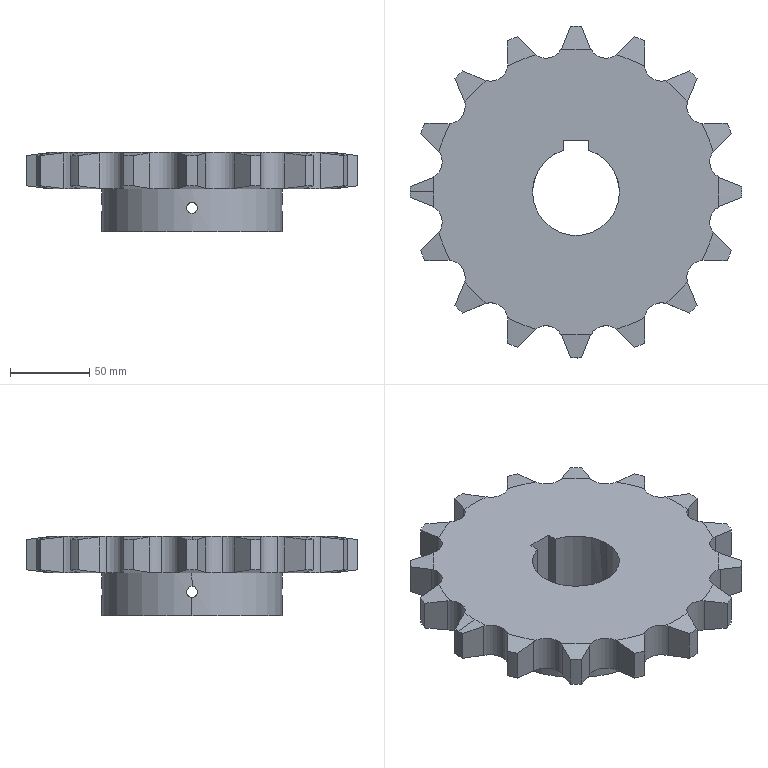Part | STEP file | 24A16T (motor sprocket) | 1 solid | 124 faces | box 210 x 210 x 50 mm | volume 787504 mm3 | cylinder 52 | plane 38 | cone 34 | commonest cylinder face diameters 22 x22 210 x17 6.8 x8 55 x3 114 x2